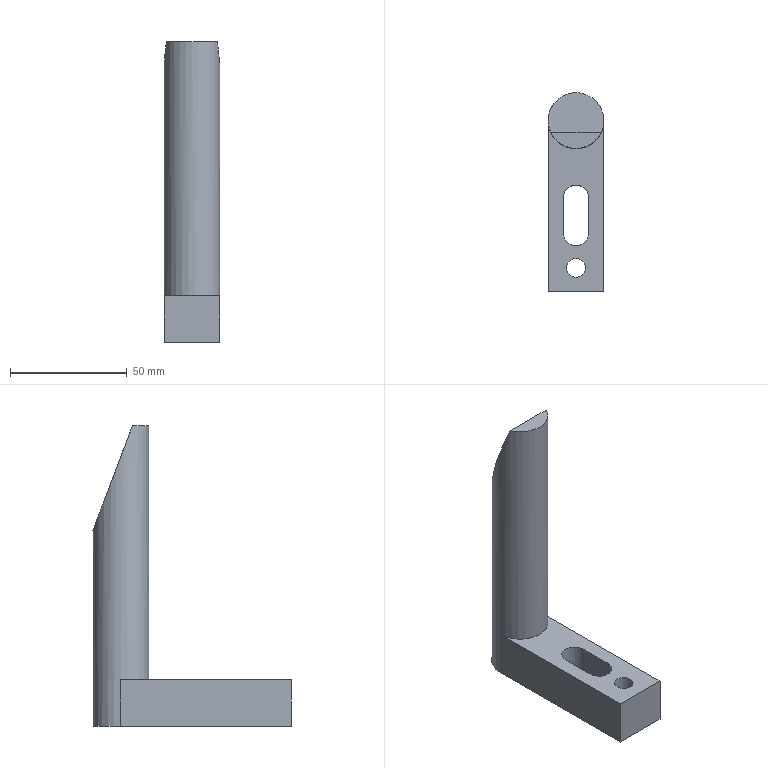Part | NX | features MAIN_BODY 2 | 1 solid | 13 faces | box 24 x 85 x 129 mm | volume 75843 mm3 | plane 9 | cylinder 4 | commonest cylinder face diameters 11 x2 8 x1 24 x1
STEP:
#1=CARTESIAN_POINT('',(-690.,-575.,-120.));
#2=VERTEX_POINT('',#1);
#3=CARTESIAN_POINT('',(-714.,-575.,-120.));
#4=VERTEX_POINT('',#3);
#5=CARTESIAN_POINT('',(-702.,-575.,-120.));
#6=DIRECTION('',(0.,0.,1.));
#7=DIRECTION('',(1.,0.,0.));
#8=AXIS2_PLACEMENT_3D('',#5,#6,#7);
#9=CIRCLE('',#8,12.);
#10=EDGE_CURVE('',#2,#4,#9,.T.);
#11=ORIENTED_EDGE('',*,*,#10,.T.);
#12=CARTESIAN_POINT('',(-714.,-575.,-100.));
#13=VERTEX_POINT('',#12);
#14=CARTESIAN_POINT('',(-714.,-575.,-76.));
#15=DIRECTION('',(0.,0.,-1.));
#16=VECTOR('',#15,1000.);
#17=LINE('',#14,#16);
#18=EDGE_CURVE('',#13,#4,#17,.T.);
#19=ORIENTED_EDGE('',*,*,#18,.F.);
#20=CARTESIAN_POINT('',(-690.,-575.,-100.));
#21=VERTEX_POINT('',#20);
#22=CARTESIAN_POINT('',(-702.,-575.,-100.));
#23=DIRECTION('',(0.,0.,1.));
#24=DIRECTION('',(1.,0.,0.));
#25=AXIS2_PLACEMENT_3D('',#22,#23,#24);
#26=CIRCLE('',#25,12.);
#27=EDGE_CURVE('',#21,#13,#26,.F.);
#28=ORIENTED_EDGE('',*,*,#27,.F.);
#29=CARTESIAN_POINT('',(-690.,-575.,-76.));
#30=DIRECTION('',(0.,0.,-1.));
#31=VECTOR('',#30,1000.);
#32=LINE('',#29,#31);
#33=EDGE_CURVE('',#21,#2,#32,.T.);
#34=ORIENTED_EDGE('',*,*,#33,.T.);
#35=EDGE_LOOP('',(#11,#19,#28,#34));
#36=FACE_BOUND('',#35,.T.);
#37=CARTESIAN_POINT('',(-691.091,-580.,9.));
#38=VERTEX_POINT('',#37);
#39=CARTESIAN_POINT('',(-712.909,-580.,9.));
#40=VERTEX_POINT('',#39);
#41=CARTESIAN_POINT('',(-702.,-575.,-4.235));
#42=DIRECTION('',(0.,0.9355,0.3534));
#43=DIRECTION('',(0.,0.3534,-0.9355));
#44=AXIS2_PLACEMENT_3D('',#41,#42,#43);
#45=ELLIPSE('',#44,33.956,12.);
#46=EDGE_CURVE('',#38,#40,#45,.T.);
#47=ORIENTED_EDGE('',*,*,#46,.F.);
#48=CARTESIAN_POINT('',(-702.,-575.,9.));
#49=DIRECTION('',(0.,0.,1.));
#50=DIRECTION('',(1.,0.,0.));
#51=AXIS2_PLACEMENT_3D('',#48,#49,#50);
#52=CIRCLE('',#51,12.);
#53=EDGE_CURVE('',#40,#38,#52,.T.);
#54=ORIENTED_EDGE('',*,*,#53,.F.);
#55=EDGE_LOOP('',(#47,#54));
#56=FACE_BOUND('',#55,.T.);
#57=CARTESIAN_POINT('',(-702.,-575.,4.));
#58=DIRECTION('',(0.,0.,-1.));
#59=DIRECTION('',(-1.,0.,0.));
#60=AXIS2_PLACEMENT_3D('',#57,#58,#59);
#61=CYLINDRICAL_SURFACE('',#60,12.);
#62=ADVANCED_FACE('',(#36,#56),#61,.T.);
#63=ORIENTED_EDGE('',*,*,#53,.T.);
#64=CARTESIAN_POINT('',(-702.,-580.,9.));
#65=DIRECTION('',(-1.,0.,0.));
#66=VECTOR('',#65,1000.);
#67=LINE('',#64,#66);
#68=EDGE_CURVE('',#38,#40,#67,.T.);
#69=ORIENTED_EDGE('',*,*,#68,.T.);
#70=EDGE_LOOP('',(#63,#69));
#71=FACE_BOUND('',#70,.T.);
#72=CARTESIAN_POINT('',(-702.,-575.,9.));
#73=DIRECTION('',(0.,0.,1.));
#74=DIRECTION('',(1.,0.,0.));
#75=AXIS2_PLACEMENT_3D('',#72,#73,#74);
#76=PLANE('',#75);
#77=ADVANCED_FACE('',(#71),#76,.T.);
#78=CARTESIAN_POINT('',(-706.,-638.,-100.));
#79=VERTEX_POINT('',#78);
#80=CARTESIAN_POINT('',(-702.,-638.,-100.));
#81=DIRECTION('',(0.,0.,-1.));
#82=DIRECTION('',(-1.,0.,0.));
#83=AXIS2_PLACEMENT_3D('',#80,#81,#82);
#84=CIRCLE('',#83,4.);
#85=EDGE_CURVE('',#79,#79,#84,.T.);
#86=ORIENTED_EDGE('',*,*,#85,.T.);
#87=EDGE_LOOP('',(#86));
#88=FACE_BOUND('',#87,.T.);
#89=CARTESIAN_POINT('',(-707.5,-623.,-100.));
#90=VERTEX_POINT('',#89);
#91=CARTESIAN_POINT('',(-707.5,-608.,-100.));
#92=VERTEX_POINT('',#91);
#93=CARTESIAN_POINT('',(-707.5,-623.,-100.));
#94=DIRECTION('',(0.,1.,0.));
#95=VECTOR('',#94,1000.);
#96=LINE('',#93,#95);
#97=EDGE_CURVE('',#90,#92,#96,.T.);
#98=ORIENTED_EDGE('',*,*,#97,.T.);
#99=CARTESIAN_POINT('',(-696.5,-608.,-100.));
#100=VERTEX_POINT('',#99);
#101=CARTESIAN_POINT('',(-702.,-608.,-100.));
#102=DIRECTION('',(0.,0.,1.));
#103=DIRECTION('',(1.,0.,0.));
#104=AXIS2_PLACEMENT_3D('',#101,#102,#103);
#105=CIRCLE('',#104,5.5);
#106=EDGE_CURVE('',#100,#92,#105,.T.);
#107=ORIENTED_EDGE('',*,*,#106,.F.);
#108=CARTESIAN_POINT('',(-696.5,-623.,-100.));
#109=VERTEX_POINT('',#108);
#110=CARTESIAN_POINT('',(-696.5,-623.,-100.));
#111=DIRECTION('',(0.,1.,0.));
#112=VECTOR('',#111,1000.);
#113=LINE('',#110,#112);
#114=EDGE_CURVE('',#109,#100,#113,.T.);
#115=ORIENTED_EDGE('',*,*,#114,.F.);
#116=CARTESIAN_POINT('',(-702.,-623.,-100.));
#117=DIRECTION('',(0.,0.,1.));
#118=DIRECTION('',(1.,0.,0.));
#119=AXIS2_PLACEMENT_3D('',#116,#117,#118);
#120=CIRCLE('',#119,5.5);
#121=EDGE_CURVE('',#90,#109,#120,.T.);
#122=ORIENTED_EDGE('',*,*,#121,.F.);
#123=EDGE_LOOP('',(#98,#107,#115,#122));
#124=FACE_BOUND('',#123,.T.);
#125=CARTESIAN_POINT('',(-690.,-648.,-100.));
#126=VERTEX_POINT('',#125);
#127=CARTESIAN_POINT('',(-690.,-663.,-100.));
#128=DIRECTION('',(0.,1.,0.));
#129=VECTOR('',#128,1000.);
#130=LINE('',#127,#129);
#131=EDGE_CURVE('',#126,#21,#130,.T.);
#132=ORIENTED_EDGE('',*,*,#131,.T.);
#133=ORIENTED_EDGE('',*,*,#27,.T.);
#134=CARTESIAN_POINT('',(-714.,-648.,-100.));
#135=VERTEX_POINT('',#134);
#136=CARTESIAN_POINT('',(-714.,-575.,-100.));
#137=DIRECTION('',(0.,-1.,0.));
#138=VECTOR('',#137,1000.);
#139=LINE('',#136,#138);
#140=EDGE_CURVE('',#13,#135,#139,.T.);
#141=ORIENTED_EDGE('',*,*,#140,.T.);
#142=CARTESIAN_POINT('',(-714.,-648.,-100.));
#143=DIRECTION('',(1.,0.,0.));
#144=VECTOR('',#143,1000.);
#145=LINE('',#142,#144);
#146=EDGE_CURVE('',#135,#126,#145,.T.);
#147=ORIENTED_EDGE('',*,*,#146,.T.);
#148=EDGE_LOOP('',(#132,#133,#141,#147));
#149=FACE_BOUND('',#148,.T.);
#150=CARTESIAN_POINT('',(-714.,-575.,-100.));
#151=DIRECTION('',(0.,0.,1.));
#152=DIRECTION('',(1.,0.,0.));
#153=AXIS2_PLACEMENT_3D('',#150,#151,#152);
#154=PLANE('',#153);
#155=ADVANCED_FACE('',(#88,#124,#149),#154,.T.);
#156=CARTESIAN_POINT('',(-714.,-648.,-120.));
#157=VERTEX_POINT('',#156);
#158=CARTESIAN_POINT('',(-714.,-575.,-120.));
#159=DIRECTION('',(0.,-1.,0.));
#160=VECTOR('',#159,1000.);
#161=LINE('',#158,#160);
#162=EDGE_CURVE('',#4,#157,#161,.T.);
#163=ORIENTED_EDGE('',*,*,#162,.T.);
#164=CARTESIAN_POINT('',(-714.,-648.,-76.));
#165=DIRECTION('',(0.,0.,-1.));
#166=VECTOR('',#165,1000.);
#167=LINE('',#164,#166);
#168=EDGE_CURVE('',#135,#157,#167,.T.);
#169=ORIENTED_EDGE('',*,*,#168,.F.);
#170=ORIENTED_EDGE('',*,*,#140,.F.);
#171=ORIENTED_EDGE('',*,*,#18,.T.);
#172=EDGE_LOOP('',(#163,#169,#170,#171));
#173=FACE_BOUND('',#172,.T.);
#174=CARTESIAN_POINT('',(-714.,-575.,-76.));
#175=DIRECTION('',(1.,0.,0.));
#176=DIRECTION('',(0.,1.,0.));
#177=AXIS2_PLACEMENT_3D('',#174,#175,#176);
#178=PLANE('',#177);
#179=ADVANCED_FACE('',(#173),#178,.F.);
#180=CARTESIAN_POINT('',(-690.,-648.,-120.));
#181=VERTEX_POINT('',#180);
#182=CARTESIAN_POINT('',(-714.,-648.,-120.));
#183=DIRECTION('',(1.,0.,0.));
#184=VECTOR('',#183,1000.);
#185=LINE('',#182,#184);
#186=EDGE_CURVE('',#157,#181,#185,.T.);
#187=ORIENTED_EDGE('',*,*,#186,.T.);
#188=CARTESIAN_POINT('',(-690.,-648.,-76.));
#189=DIRECTION('',(0.,0.,-1.));
#190=VECTOR('',#189,1000.);
#191=LINE('',#188,#190);
#192=EDGE_CURVE('',#126,#181,#191,.T.);
#193=ORIENTED_EDGE('',*,*,#192,.F.);
#194=ORIENTED_EDGE('',*,*,#146,.F.);
#195=ORIENTED_EDGE('',*,*,#168,.T.);
#196=EDGE_LOOP('',(#187,#193,#194,#195));
#197=FACE_BOUND('',#196,.T.);
#198=CARTESIAN_POINT('',(-714.,-648.,-76.));
#199=DIRECTION('',(0.,1.,0.));
#200=DIRECTION('',(0.,0.,1.));
#201=AXIS2_PLACEMENT_3D('',#198,#199,#200);
#202=PLANE('',#201);
#203=ADVANCED_FACE('',(#197),#202,.F.);
#204=CARTESIAN_POINT('',(-690.,-663.,-120.));
#205=DIRECTION('',(0.,1.,0.));
#206=VECTOR('',#205,1000.);
#207=LINE('',#204,#206);
#208=EDGE_CURVE('',#181,#2,#207,.T.);
#209=ORIENTED_EDGE('',*,*,#208,.T.);
#210=ORIENTED_EDGE('',*,*,#33,.F.);
#211=ORIENTED_EDGE('',*,*,#131,.F.);
#212=ORIENTED_EDGE('',*,*,#192,.T.);
#213=EDGE_LOOP('',(#209,#210,#211,#212));
#214=FACE_BOUND('',#213,.T.);
#215=CARTESIAN_POINT('',(-690.,-663.,-76.));
#216=DIRECTION('',(-1.,0.,0.));
#217=DIRECTION('',(0.,-1.,0.));
#218=AXIS2_PLACEMENT_3D('',#215,#216,#217);
#219=PLANE('',#218);
#220=ADVANCED_FACE('',(#214),#219,.F.);
#221=CARTESIAN_POINT('',(-706.,-638.,-120.));
#222=VERTEX_POINT('',#221);
#223=CARTESIAN_POINT('',(-702.,-638.,-120.));
#224=DIRECTION('',(0.,0.,-1.));
#225=DIRECTION('',(-1.,0.,0.));
#226=AXIS2_PLACEMENT_3D('',#223,#224,#225);
#227=CIRCLE('',#226,4.);
#228=EDGE_CURVE('',#222,#222,#227,.T.);
#229=ORIENTED_EDGE('',*,*,#228,.F.);
#230=EDGE_LOOP('',(#229));
#231=FACE_BOUND('',#230,.T.);
#232=CARTESIAN_POINT('',(-696.5,-608.,-120.));
#233=VERTEX_POINT('',#232);
#234=CARTESIAN_POINT('',(-707.5,-608.,-120.));
#235=VERTEX_POINT('',#234);
#236=CARTESIAN_POINT('',(-702.,-608.,-120.));
#237=DIRECTION('',(0.,0.,1.));
#238=DIRECTION('',(1.,0.,0.));
#239=AXIS2_PLACEMENT_3D('',#236,#237,#238);
#240=CIRCLE('',#239,5.5);
#241=EDGE_CURVE('',#233,#235,#240,.T.);
#242=ORIENTED_EDGE('',*,*,#241,.T.);
#243=CARTESIAN_POINT('',(-707.5,-623.,-120.));
#244=VERTEX_POINT('',#243);
#245=CARTESIAN_POINT('',(-707.5,-638.,-120.));
#246=DIRECTION('',(0.,1.,0.));
#247=VECTOR('',#246,1000.);
#248=LINE('',#245,#247);
#249=EDGE_CURVE('',#244,#235,#248,.T.);
#250=ORIENTED_EDGE('',*,*,#249,.F.);
#251=CARTESIAN_POINT('',(-696.5,-623.,-120.));
#252=VERTEX_POINT('',#251);
#253=CARTESIAN_POINT('',(-702.,-623.,-120.));
#254=DIRECTION('',(0.,0.,1.));
#255=DIRECTION('',(1.,0.,0.));
#256=AXIS2_PLACEMENT_3D('',#253,#254,#255);
#257=CIRCLE('',#256,5.5);
#258=EDGE_CURVE('',#244,#252,#257,.T.);
#259=ORIENTED_EDGE('',*,*,#258,.T.);
#260=CARTESIAN_POINT('',(-696.5,-638.,-120.));
#261=DIRECTION('',(0.,1.,0.));
#262=VECTOR('',#261,1000.);
#263=LINE('',#260,#262);
#264=EDGE_CURVE('',#252,#233,#263,.T.);
#265=ORIENTED_EDGE('',*,*,#264,.T.);
#266=EDGE_LOOP('',(#242,#250,#259,#265));
#267=FACE_BOUND('',#266,.T.);
#268=ORIENTED_EDGE('',*,*,#162,.F.);
#269=ORIENTED_EDGE('',*,*,#10,.F.);
#270=ORIENTED_EDGE('',*,*,#208,.F.);
#271=ORIENTED_EDGE('',*,*,#186,.F.);
#272=EDGE_LOOP('',(#268,#269,#270,#271));
#273=FACE_BOUND('',#272,.T.);
#274=CARTESIAN_POINT('',(-714.,-575.,-120.));
#275=DIRECTION('',(0.,0.,1.));
#276=DIRECTION('',(1.,0.,0.));
#277=AXIS2_PLACEMENT_3D('',#274,#275,#276);
#278=PLANE('',#277);
#279=ADVANCED_FACE('',(#231,#267,#273),#278,.F.);
#280=ORIENTED_EDGE('',*,*,#68,.F.);
#281=ORIENTED_EDGE('',*,*,#46,.T.);
#282=EDGE_LOOP('',(#280,#281));
#283=FACE_BOUND('',#282,.T.);
#284=CARTESIAN_POINT('',(-773.5,-580.,9.));
#285=DIRECTION('',(0.,0.9355,0.3534));
#286=DIRECTION('',(0.,-0.3534,0.9355));
#287=AXIS2_PLACEMENT_3D('',#284,#285,#286);
#288=PLANE('',#287);
#289=ADVANCED_FACE('',(#283),#288,.T.);
#290=ORIENTED_EDGE('',*,*,#97,.F.);
#291=CARTESIAN_POINT('',(-707.5,-623.,-76.));
#292=DIRECTION('',(0.,0.,1.));
#293=VECTOR('',#292,1000.);
#294=LINE('',#291,#293);
#295=EDGE_CURVE('',#244,#90,#294,.T.);
#296=ORIENTED_EDGE('',*,*,#295,.F.);
#297=ORIENTED_EDGE('',*,*,#249,.T.);
#298=CARTESIAN_POINT('',(-707.5,-608.,-76.));
#299=DIRECTION('',(0.,0.,1.));
#300=VECTOR('',#299,1000.);
#301=LINE('',#298,#300);
#302=EDGE_CURVE('',#235,#92,#301,.T.);
#303=ORIENTED_EDGE('',*,*,#302,.T.);
#304=EDGE_LOOP('',(#290,#296,#297,#303));
#305=FACE_BOUND('',#304,.T.);
#306=CARTESIAN_POINT('',(-707.5,-623.,-76.));
#307=DIRECTION('',(-1.,0.,0.));
#308=DIRECTION('',(0.,0.,1.));
#309=AXIS2_PLACEMENT_3D('',#306,#307,#308);
#310=PLANE('',#309);
#311=ADVANCED_FACE('',(#305),#310,.F.);
#312=ORIENTED_EDGE('',*,*,#121,.T.);
#313=CARTESIAN_POINT('',(-696.5,-623.,-76.));
#314=DIRECTION('',(0.,0.,1.));
#315=VECTOR('',#314,1000.);
#316=LINE('',#313,#315);
#317=EDGE_CURVE('',#252,#109,#316,.T.);
#318=ORIENTED_EDGE('',*,*,#317,.F.);
#319=ORIENTED_EDGE('',*,*,#258,.F.);
#320=ORIENTED_EDGE('',*,*,#295,.T.);
#321=EDGE_LOOP('',(#312,#318,#319,#320));
#322=FACE_BOUND('',#321,.T.);
#323=CARTESIAN_POINT('',(-702.,-623.,-76.));
#324=DIRECTION('',(0.,0.,1.));
#325=DIRECTION('',(1.,0.,0.));
#326=AXIS2_PLACEMENT_3D('',#323,#324,#325);
#327=CYLINDRICAL_SURFACE('',#326,5.5);
#328=ADVANCED_FACE('',(#322),#327,.F.);
#329=ORIENTED_EDGE('',*,*,#114,.T.);
#330=CARTESIAN_POINT('',(-696.5,-608.,-76.));
#331=DIRECTION('',(0.,0.,1.));
#332=VECTOR('',#331,1000.);
#333=LINE('',#330,#332);
#334=EDGE_CURVE('',#233,#100,#333,.T.);
#335=ORIENTED_EDGE('',*,*,#334,.F.);
#336=ORIENTED_EDGE('',*,*,#264,.F.);
#337=ORIENTED_EDGE('',*,*,#317,.T.);
#338=EDGE_LOOP('',(#329,#335,#336,#337));
#339=FACE_BOUND('',#338,.T.);
#340=CARTESIAN_POINT('',(-696.5,-623.,-76.));
#341=DIRECTION('',(1.,0.,0.));
#342=DIRECTION('',(0.,0.,-1.));
#343=AXIS2_PLACEMENT_3D('',#340,#341,#342);
#344=PLANE('',#343);
#345=ADVANCED_FACE('',(#339),#344,.F.);
#346=ORIENTED_EDGE('',*,*,#106,.T.);
#347=ORIENTED_EDGE('',*,*,#302,.F.);
#348=ORIENTED_EDGE('',*,*,#241,.F.);
#349=ORIENTED_EDGE('',*,*,#334,.T.);
#350=EDGE_LOOP('',(#346,#347,#348,#349));
#351=FACE_BOUND('',#350,.T.);
#352=CARTESIAN_POINT('',(-702.,-608.,-76.));
#353=DIRECTION('',(0.,0.,1.));
#354=DIRECTION('',(1.,0.,0.));
#355=AXIS2_PLACEMENT_3D('',#352,#353,#354);
#356=CYLINDRICAL_SURFACE('',#355,5.5);
#357=ADVANCED_FACE('',(#351),#356,.F.);
#358=ORIENTED_EDGE('',*,*,#228,.T.);
#359=EDGE_LOOP('',(#358));
#360=FACE_BOUND('',#359,.T.);
#361=ORIENTED_EDGE('',*,*,#85,.F.);
#362=EDGE_LOOP('',(#361));
#363=FACE_BOUND('',#362,.T.);
#364=CARTESIAN_POINT('',(-702.,-638.,-76.));
#365=DIRECTION('',(0.,0.,-1.));
#366=DIRECTION('',(-1.,0.,0.));
#367=AXIS2_PLACEMENT_3D('',#364,#365,#366);
#368=CYLINDRICAL_SURFACE('',#367,4.);
#369=ADVANCED_FACE('',(#360,#363),#368,.F.);
#370=CLOSED_SHELL('',(#62,#77,#155,#179,#203,#220,#279,#289,#311,#328,#345,#357,#369));
#371=MANIFOLD_SOLID_BREP('',#370);
#372=(LENGTH_UNIT()NAMED_UNIT(*)SI_UNIT(.MILLI.,.METRE.));
#373=UNCERTAINTY_MEASURE_WITH_UNIT(LENGTH_MEASURE(0.00001),#372,'','');
#374=(NAMED_UNIT(*)PLANE_ANGLE_UNIT()SI_UNIT($,.RADIAN.));
#375=(NAMED_UNIT(*)SI_UNIT($,.STERADIAN.)SOLID_ANGLE_UNIT());
#376=(GEOMETRIC_REPRESENTATION_CONTEXT(3)GLOBAL_UNCERTAINTY_ASSIGNED_CONTEXT((#373))GLOBAL_UNIT_ASSIGNED_CONTEXT((#372,#374,#375))REPRESENTATION_CONTEXT('',''));
#377=ADVANCED_BREP_SHAPE_REPRESENTATION('',(#371),#376);